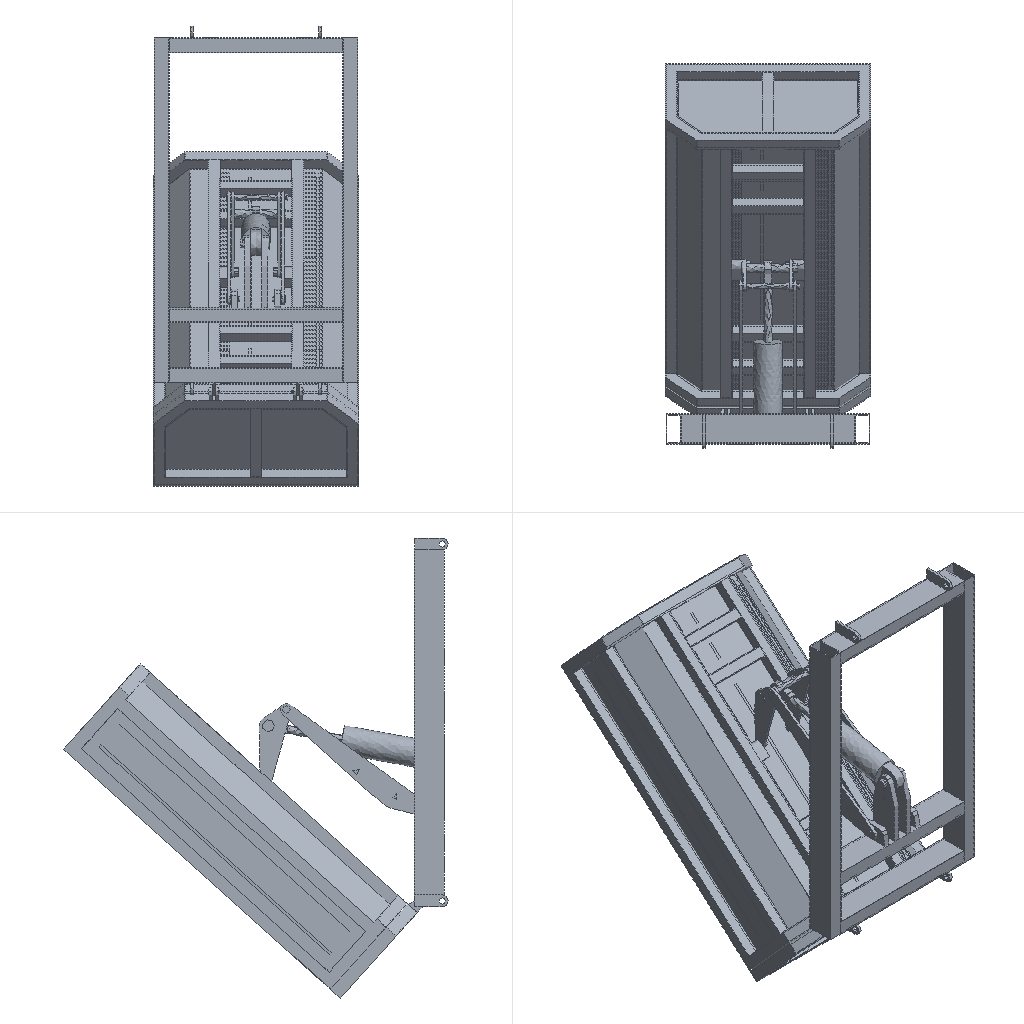Simulation study | ansys workbench
Ansys APDL input file, long lists of numbers shortened:
/batch
/config,noeldb,1     ! force off writing results to database
*get,_wallstrt,active,,time,wall
! ANSYS input file written by Workbench version 2022 R1
! File used for geometry attach:
/title,wbnew--____ (B5)
! ****** Begin Custom Load Command Snippet ******
/COM, ACT Extensions:
/COM,     LSDYNA, 2021.1
/COM,
! ****** End   Custom Load Command Snippet ******
*DIM,_wb_ProjectScratch_dir,string,248
_wb_ProjectScratch_dir(1) = ''
*DIM,_wb_SolverFiles_dir,string,248
_wb_SolverFiles_dir(1) = ''
*DIM,_wb_userfiles_dir,string,248
_wb_userfiles_dir(1) = ''
/com,--- Data in consistent NMM units. See Solving Units in the help system for more information.
/units,MPA
/nopr
/wb,file,start              !  signify a WB generated input file
/prep7
! Turn off shape checking because checks already performed inside WB mesher.
! See help system for more information.
SHPP,OFF,,NOWARN
/nolist
etcon,set             ! allow ANSYS to choose best KEYOP's for 180x elements, resets any applicable keyopt to MAPDL defaults
/com,*********** Nodes for the whole assembly ***********
nblock,3,,263278
(1i9,3e20.9e3)
        1    -2.353006712E+02    -4.029652814E+01    -6.964386465E+02
! (239343 more lines like these left out)
-1
/com,*********** Nodes for all Remote Points ***********
nblock,3
(1i9,3e20.9e3)
   239345    -1.888006686E+02     4.073828789E+02    -9.568132104E+02
-1
/wb,elem,start            !  set before creation of elements
/com,*********** Elements for Body 1 "__\____-____1" ***********
et,1,186
keyo,1,2,1          ! set full integration on SOLID186
eblock,19,solid,,8004
(19i9)
        1        1        1        1        0        0        0        0       20        0    13307    32471    32472    34084    34085    33944    33943    35521    35520
! (16007 more lines like these left out)
-1
/com,*********** Elements for Body 2 "______3c_____3e_\__________________(gb t6728-2002) 40__3(1)[6]" ***********
et,2,187
eblock,19,solid,,10404
(19i9)
        2        2        2        2        0        0        0        0       10        0     2903     6093     8090     9264     8092    10282    22392    10284    10283
! (20807 more lines like these left out)
-1
/com,*********** Elements for Body 3 "__2\____1" ***********
et,3,186
keyo,3,2,1          ! set full integration on SOLID186
eblock,19,solid,,129
(19i9)
        3        3        3        3        0        0        0        0       20        0    98906   231933   231934   231961   231960   232046   232045   232018   232019
! (257 more lines like these left out)
-1
/com,*********** Elements for Body 4 "__2\____1" ***********
et,4,186
keyo,4,2,1          ! set full integration on SOLID186
eblock,19,solid,,129
(19i9)
        4        4        4        4        0        0        0        0       20        0    99035   233038   233039   233066   233065   233151   233150   233123   233124
! (257 more lines like these left out)
-1
/com,*********** Elements for Body 5 "__28__250\____-____2" ***********
et,5,187
eblock,19,solid,,1867
(19i9)
        5        5        5        5        0        0        0        0       10        0      284      779     1143     1250     1242     2117     3926     2120     2119
! (3733 more lines like these left out)
-1
! (19 more sections like these left out)
/wb,elem,end               !  done creating elements
/com,*********** Send User Defined Coordinate System(s) ***********
csys,0
toffst,273.15,  ! Temperature offset from absolute zero
/com,*********** Set Reference Temperature ***********
tref,22.
/wb,mat,start              !  starting to send materials
/com,*********** Send Materials ***********
Temperature = 'TEMP' ! Temperature
MP,DENS,1,7.85e-09,	! tonne mm^-3
MP,ALPX,1,1.2e-05,	! C^-1
MP,C,1,434000000,	! mm^2 s^-2 C^-1
MP,KXX,1,60.5,	! tonne mm s^-3 C^-1
MP,RSVX,1,0.00017,	! ohm mm
MP,EX,1,200000,	! tonne s^-2 mm^-1
MP,NUXY,1,0.3,
MP,MURX,1,10000,
Temperature = 'TEMP' ! Temperature
MP,DENS,2,7.85e-09,	! tonne mm^-3
MP,ALPX,2,1.2e-05,	! C^-1
MP,C,2,434000000,	! mm^2 s^-2 C^-1
MP,KXX,2,60.5,	! tonne mm s^-3 C^-1
MP,RSVX,2,0.00017,	! ohm mm
MP,EX,2,200000,	! tonne s^-2 mm^-1
MP,NUXY,2,0.3,
MP,MURX,2,10000,
Temperature = 'TEMP' ! Temperature
MP,DENS,3,7.85e-09,	! tonne mm^-3
MP,ALPX,3,1.2e-05,	! C^-1
MP,C,3,434000000,	! mm^2 s^-2 C^-1
MP,KXX,3,60.5,	! tonne mm s^-3 C^-1
MP,RSVX,3,0.00017,	! ohm mm
MP,EX,3,200000,	! tonne s^-2 mm^-1
MP,NUXY,3,0.3,
MP,MURX,3,10000,
Temperature = 'TEMP' ! Temperature
MP,DENS,4,7.85e-09,	! tonne mm^-3
MP,ALPX,4,1.2e-05,	! C^-1
MP,C,4,434000000,	! mm^2 s^-2 C^-1
MP,KXX,4,60.5,	! tonne mm s^-3 C^-1
MP,RSVX,4,0.00017,	! ohm mm
MP,EX,4,200000,	! tonne s^-2 mm^-1
MP,NUXY,4,0.3,
MP,MURX,4,10000,
Temperature = 'TEMP' ! Temperature
MP,DENS,5,7.85e-09,	! tonne mm^-3
MP,ALPX,5,1.2e-05,	! C^-1
MP,C,5,434000000,	! mm^2 s^-2 C^-1
MP,KXX,5,60.5,	! tonne mm s^-3 C^-1
MP,RSVX,5,0.00017,	! ohm mm
MP,EX,5,200000,	! tonne s^-2 mm^-1
MP,NUXY,5,0.3,
MP,MURX,5,10000,
Temperature = 'TEMP' ! Temperature
MP,DENS,6,7.85e-09,	! tonne mm^-3
MP,ALPX,6,1.2e-05,	! C^-1
MP,C,6,434000000,	! mm^2 s^-2 C^-1
MP,KXX,6,60.5,	! tonne mm s^-3 C^-1
MP,RSVX,6,0.00017,	! ohm mm
MP,EX,6,200000,	! tonne s^-2 mm^-1
MP,NUXY,6,0.3,
MP,MURX,6,10000,
Temperature = 'TEMP' ! Temperature
MP,DENS,7,7.85e-09,	! tonne mm^-3
MP,ALPX,7,1.2e-05,	! C^-1
MP,C,7,434000000,	! mm^2 s^-2 C^-1
MP,KXX,7,60.5,	! tonne mm s^-3 C^-1
MP,RSVX,7,0.00017,	! ohm mm
MP,EX,7,200000,	! tonne s^-2 mm^-1
MP,NUXY,7,0.3,
MP,MURX,7,10000,
Temperature = 'TEMP' ! Temperature
MP,DENS,8,7.85e-09,	! tonne mm^-3
MP,ALPX,8,1.2e-05,	! C^-1
MP,C,8,434000000,	! mm^2 s^-2 C^-1
MP,KXX,8,60.5,	! tonne mm s^-3 C^-1
MP,RSVX,8,0.00017,	! ohm mm
MP,EX,8,200000,	! tonne s^-2 mm^-1
MP,NUXY,8,0.3,
MP,MURX,8,10000,
Temperature = 'TEMP' ! Temperature
MP,DENS,9,7.85e-09,	! tonne mm^-3
MP,ALPX,9,1.2e-05,	! C^-1
MP,C,9,434000000,	! mm^2 s^-2 C^-1
MP,KXX,9,60.5,	! tonne mm s^-3 C^-1
MP,RSVX,9,0.00017,	! ohm mm
MP,EX,9,200000,	! tonne s^-2 mm^-1
! (137 more lines like these left out)
/wb,mat,end                !  done sending materials
!************************* Model Summary ********************
!__\____-____1,	结构钢,	matid,	1
!______3c_____3e_\__________________(gb t6728-2002) 40__3(1)[6],	结构钢,	matid,	2
!__2\____1,	结构钢,	matid,	3
!__2\____1,	结构钢,	matid,	4
!__28__250\____-____2,	结构钢,	matid,	5
!__3\____-____5,	结构钢,	matid,	6
!__3\____-____5,	结构钢,	matid,	7
!__1\____-____1,	结构钢,	matid,	8
!__1\____-____1,	结构钢,	matid,	9
!________3c_____3e_\__________________gb_Mt6728-2002 100__50__3(1)[2],	结构钢,	matid,	10
!____1\____1,	结构钢,	matid,	11
!____1\____1,	结构钢,	matid,	12
!____2\______1,	结构钢,	matid,	13
!____2\______1,	结构钢,	matid,	14
!M30X90\____-____1,	结构钢,	matid,	15
!M20X40__\____-____1,	结构钢,	matid,	16
!M20X40__\____-____1,	结构钢,	matid,	17
!M20X200__\____-____1,	结构钢,	matid,	18
!M30X180__\____-____1,	结构钢,	matid,	19
!M20X20-16____\____1,	结构钢,	matid,	20
!M20X20-16____\____1,	结构钢,	matid,	21
!M12X38__\____-____1,	结构钢,	matid,	22
!M12X38__\____-____1,	结构钢,	matid,	23
!______3c_____3e_\__________________(gb t6728-2002) 40__3(1)[1],	结构钢,	matid,	24
!************************* End Model Summary ********************
! get the diagonal of the bounding box. Needed later for other things
*get,_xmin,node,,mnloc,x
*get,_ymin,node,,mnloc,y
*get,_zmin,node,,mnloc,z
*get,_xmax,node,,mxloc,x
*get,_ymax,node,,mxloc,y
*get,_zmax,node,,mxloc,z
_ASMDIAG=(_xmax-_xmin)*(_xmax-_xmin)+(_ymax-_ymin)*(_ymax-_ymin)+(_zmax-_zmin)*(_zmax-_zmin)
_ASMDIAG=SQRT(_ASMDIAG)
/wb,contact,start          !  starting to send contact
/com,*********** Create Contact "接触区域" ***********
/com,            Real Constant Set For Above Contact Is 26 & 25
*set,tid,26
*set,cid,25
r,tid
r,cid
et,tid,170
et,cid,174
eblock,10,,,138
(15i9)
   176923       26       26       26        0    33942    35521    33943    33943    64183    64185    33943    64182
! (137 more lines like these left out)
-1
eblock,10,,,138
(15i9)
   177061       25       25       25        0    33942    35521    33943    33943    64183    64185    33943    64182
! (137 more lines like these left out)
-1
eblock,10,,,162
(15i9)
   177199       25       26       25        0     8144     8214     8175     8175    22993    23314     8175    22991
! (161 more lines like these left out)
-1
eblock,10,,,162
(15i9)
   177361       26       25       26        0     8144     8214     8175     8175    22993    23314     8175    22991
! (161 more lines like these left out)
-1
keyo,cid,8,2               ! auto create asymmetric contact (from Program Controlled setting)
keyo,cid,10,0              ! adjust contact stiffness each NR iteration (from Program Controlled setting)
keyo,cid,12,5              ! bonded always
keyo,cid,2,2               ! MPC contact.  Valid only for bonded or no separation.  Requires nodal detection
keyo,cid,4,2               ! on nodal point - normal to target surface (from Program Controlled setting)
keyo,cid,9,1               ! ignore initial gaps/penetration
keyo,cid,7,0               ! No Prediction
rmod,tid,3,10.      ! FKN
rmod,tid,5,0.       ! ICONT
rmod,tid,6,-5.      ! PINB
rmod,tid,10,0.      ! CNOF
rmod,tid,12,0.      ! FKT
rmod,tid,36,95      ! WB DSID
rmod,cid,3,10.      ! FKN
rmod,cid,5,0.       ! ICONT
rmod,cid,6,-5.      ! PINB
rmod,cid,10,0.      ! CNOF
rmod,cid,12,0.      ! FKT
rmod,cid,36,95      ! WB DSID
/com,*********** Create Contact "接触区域 8" ***********
/com,            Real Constant Set For Above Contact Is 28 & 27
*set,tid,28
*set,cid,27
r,tid
r,cid
et,tid,170
et,cid,174
eblock,10,,,3771
(15i9)
   177523       28       28       28        0    28251    26712    26655    26654    41903    41789    41786    41787
! (3770 more lines like these left out)
-1
eblock,10,,,3771
(15i9)
   181294       27       27       27        0    28251    26712    26655    26654    41903    41789    41786    41787
! (3770 more lines like these left out)
-1
eblock,10,,,3247
(15i9)
   185065       27       28       27        0   139835   149281   144474   144474   166900   201084   144474   166896
! (3246 more lines like these left out)
-1
eblock,10,,,3247
(15i9)
   188312       28       27       28        0   139835   149281   144474   144474   166900   201084   144474   166896
! (3246 more lines like these left out)
-1
keyo,cid,8,2               ! auto create asymmetric contact (from Program Controlled setting)
keyo,cid,10,0              ! adjust contact stiffness each NR iteration (from Program Controlled setting)
keyo,cid,12,5              ! bonded always
keyo,cid,2,2               ! MPC contact.  Valid only for bonded or no separation.  Requires nodal detection
keyo,cid,4,2               ! on nodal point - normal to target surface (from Program Controlled setting)
keyo,cid,9,1               ! ignore initial gaps/penetration
keyo,cid,7,0               ! No Prediction
rmod,tid,3,10.      ! FKN
rmod,tid,5,0.       ! ICONT
rmod,tid,6,-5.      ! PINB
rmod,tid,10,0.      ! CNOF
rmod,tid,12,0.      ! FKT
rmod,tid,36,116     ! WB DSID
rmod,cid,3,10.      ! FKN
rmod,cid,5,0.       ! ICONT
rmod,cid,6,-5.      ! PINB
rmod,cid,10,0.      ! CNOF
rmod,cid,12,0.      ! FKT
rmod,cid,36,116     ! WB DSID
/com,*********** Create Contact "接触区域 11" ***********
/com,            Real Constant Set For Above Contact Is 30 & 29
*set,tid,30
*set,cid,29
r,tid
r,cid
et,tid,170
et,cid,174
eblock,10,,,54
(15i9)
   191559       30       30       30        0     6070     6066     6058     6058    10162    10117     6058    10118
! (53 more lines like these left out)
-1
eblock,10,,,54
(15i9)
   191613       29       29       29        0     6070     6066     6058     6058    10162    10117     6058    10118
! (53 more lines like these left out)
-1
eblock,10,,,96
(15i9)
   191667       29       30       29        0   238922   238921   238955   238955   239014   239016   238955   239019
! (95 more lines like these left out)
-1
eblock,10,,,96
(15i9)
   191763       30       29       30        0   238922   238921   238955   238955   239014   239016   238955   239019
! (95 more lines like these left out)
-1
keyo,cid,8,2               ! auto create asymmetric contact (from Program Controlled setting)
keyo,cid,10,0              ! adjust contact stiffness each NR iteration (from Program Controlled setting)
keyo,cid,12,5              ! bonded always
keyo,cid,2,2               ! MPC contact.  Valid only for bonded or no separation.  Requires nodal detection
keyo,cid,4,2               ! on nodal point - normal to target surface (from Program Controlled setting)
keyo,cid,9,1               ! ignore initial gaps/penetration
keyo,cid,7,0               ! No Prediction
rmod,tid,3,10.      ! FKN
rmod,tid,5,0.       ! ICONT
rmod,tid,6,-5.      ! PINB
rmod,tid,10,0.      ! CNOF
rmod,tid,12,0.      ! FKT
rmod,tid,36,125     ! WB DSID
rmod,cid,3,10.      ! FKN
rmod,cid,5,0.       ! ICONT
rmod,cid,6,-5.      ! PINB
rmod,cid,10,0.      ! CNOF
rmod,cid,12,0.      ! FKT
rmod,cid,36,125     ! WB DSID
/com,*********** Create Contact "接触区域 12" ***********
/com,            Real Constant Set For Above Contact Is 32 & 31
*set,tid,32
*set,cid,31
r,tid
r,cid
et,tid,170
et,cid,174
eblock,10,,,201
(15i9)
   191859       32       32       32        0     8144     8214     8175     8175    22993    23314     8175    22991
! (200 more lines like these left out)
-1
eblock,10,,,201
(15i9)
   192060       31       31       31        0     8144     8214     8175     8175    22993    23314     8175    22991
! (200 more lines like these left out)
-1
eblock,10,,,428
(15i9)
   192261       31       32       31        0   138273   149145   149139   149139   154407   222313   149139   154406
! (427 more lines like these left out)
-1
eblock,10,,,428
(15i9)
   192689       32       31       32        0   138273   149145   149139   149139   154407   222313   149139   154406
! (427 more lines like these left out)
-1
keyo,cid,8,2               ! auto create asymmetric contact (from Program Controlled setting)
keyo,cid,10,0              ! adjust contact stiffness each NR iteration (from Program Controlled setting)
keyo,cid,12,5              ! bonded always
keyo,cid,2,2               ! MPC contact.  Valid only for bonded or no separation.  Requires nodal detection
keyo,cid,4,2               ! on nodal point - normal to target surface (from Program Controlled setting)
keyo,cid,9,1               ! ignore initial gaps/penetration
keyo,cid,7,0               ! No Prediction
rmod,tid,3,10.      ! FKN
rmod,tid,5,0.       ! ICONT
rmod,tid,6,-5.      ! PINB
rmod,tid,10,0.      ! CNOF
rmod,tid,12,0.      ! FKT
rmod,tid,36,128     ! WB DSID
rmod,cid,3,10.      ! FKN
rmod,cid,5,0.       ! ICONT
rmod,cid,6,-5.      ! PINB
rmod,cid,10,0.      ! CNOF
rmod,cid,12,0.      ! FKT
rmod,cid,36,128     ! WB DSID
/com,*********** Create Contact "接触区域 15" ***********
/com,            Real Constant Set For Above Contact Is 34 & 33
*set,tid,34
*set,cid,33
r,tid
r,cid
et,tid,170
et,cid,174
eblock,10,,,23
(15i9)
   193117       34       34       34        0   232168   232149   232143   232167   232893   232880   232881   232925
! (22 more lines like these left out)
-1
eblock,10,,,23
(15i9)
   193140       33       33       33        0   232168   232149   232143   232167   232893   232880   232881   232925
! (22 more lines like these left out)
-1
eblock,10,,,48
(15i9)
   193163       33       34       33        0   237237   237258   237253   237253   237535   237602   237253   237534
! (47 more lines like these left out)
-1
eblock,10,,,48
(15i9)
   193211       34       33       34        0   237237   237258   237253   237253   237535   237602   237253   237534
! (47 more lines like these left out)
-1
keyo,cid,8,2               ! auto create asymmetric contact (from Program Controlled setting)
keyo,cid,10,0              ! adjust contact stiffness each NR iteration (from Program Controlled setting)
keyo,cid,12,5              ! bonded always
keyo,cid,2,2               ! MPC contact.  Valid only for bonded or no separation.  Requires nodal detection
keyo,cid,4,2               ! on nodal point - normal to target surface (from Program Controlled setting)
keyo,cid,9,1               ! ignore initial gaps/penetration
keyo,cid,7,0               ! No Prediction
rmod,tid,3,10.      ! FKN
rmod,tid,5,0.       ! ICONT
rmod,tid,6,-5.      ! PINB
rmod,tid,10,0.      ! CNOF
rmod,tid,12,0.      ! FKT
rmod,tid,36,137     ! WB DSID
rmod,cid,3,10.      ! FKN
rmod,cid,5,0.       ! ICONT
rmod,cid,6,-5.      ! PINB
rmod,cid,10,0.      ! CNOF
rmod,cid,12,0.      ! FKT
rmod,cid,36,137     ! WB DSID
! (25 more sections like these left out)
/wb,contact,end            !  done creating contacts
/golist
/wb,load,start             !  starting to send loads
/com,*********** Fixed Supports ***********
CMBLOCK,_FIXEDSU,NODE,      348
(8i10)
     78153     78154     78155     78156     78157     78158     78285     78286
! (43 more lines like these left out)
cmsel,s,_FIXEDSU
d,all,all
nsel,all
/com,*********** Create Remote Point "内部远程点" ***********
! -------- Remote Point Used by "点质量" --------
*set,tid,86
*set,cid,85
et,cid,174
et,tid,170
keyo,tid,2,1               ! Don't fix the pilot node
keyo,tid,4,000111
keyo,cid,12,5              ! Bonded Contact
keyo,cid,4,3               ! Coupled CPINTF style load
keyo,cid,2,2               ! MPC style contact
eblock,10,,,4455
(15i9)
   197199       85       85       85        0    38777    36282    38775    38776    68825    68824    73766    73767
! (4454 more lines like these left out)
-1
*set,_npilot,239345
_npilot246=_npilot
type,tid
mat ,cid
real,cid
tshape,pilo
en,201654,_npilot
tshape
/com,*********** Construct Remote Mass Using Remote Attachment ***********
*set,_tid,87
et,_tid,21           ! MASS21 element
type,_tid
mat ,_tid
real,_tid
keyo,_tid,3,2        ! 3d mass without rotary inertia
r,_tid,0.5
en,201655,239345
/gst,on,on
fini
*get,_numnode,node,0,count
*get,_numelem,elem,0,count
*get, _MAXELEMNUM, elem, 0, NUM, MAX
*get, _MAXNODENUM, node, 0, NUM, MAX
*get, _MAXELEMTYPE, etyp, 0, NUM, MAX
*get, _MAXREALCONST, real, 0, NUM, MAX
/go
/wb,load,end               !  done creating loads
/com,--- Number of total nodes = %_numnode%
/com,--- Number of contact elements = 24731
/com,--- Number of spring elements = 0
/com,--- Number of bearing elements = 0
/com,--- Number of solid elements = 100731
/com,--- Number of condensed parts = 0
/com,--- Number of total elements = %_numelem%
*get,_wallbsol,active,,time,wall
/com,****************************************************************************
/com,*************************    SOLUTION       ********************************
/com,****************************************************************************
/solu
antype,0                   ! static analysis
neqit,1,force              ! Force 1 eq iteration since only nonlinearity is bonded/no sep contact
pred,off
_thickRatio=0.208   ! Ratio of thick parts in the model
eqsl,sparse,,,,,1
cntr,print,1               ! print out contact info and also make no initial contact an error
dmpoption,emat,no             ! Don't combine emat file for DANSYS
dmpoption,esav,no             ! Don't combine esav file for DANSYS
nldiag,cont,iter           ! print out contact info each equilibrium iteration
rescontrol,,none                 ! Do not keep any restart files
/com,****************************************************
/com,******************* SOLVE FOR LS 1 OF 1 ****************
acel,0.,9806.65,0.
/nopr
/gopr
nsub,1,1,1
time,1.
outres,erase
outres,all,none
outres,nsol,all,
outres,rsol,all
outres,eangl,all
outres,etmp,all
outres,veng,all
outres,strs,all,
outres,epel,all,
outres,eppl,all,
outres,cont,all,
! *********** WB SOLVE COMMAND ***********
! check interactive state
*get,ANSINTER_,active,,int
*if,ANSINTER_,ne,0,then
/eof
*endif
solve
/com *************** Write FE CONNECTORS *********
CEWRITE,file,ce,,INTE
/com,****************************************************
/com,*************** FINISHED SOLVE FOR LS 1 *************
*get,_wallasol,active,,time,wall
/nopr
*get,_numnode,node,0,count
*get,_numelem,elem,0,count
*get, _MAXELEMNUM, elem, 0, NUM, MAX
*get, _MAXNODENUM, node, 0, NUM, MAX,,,INTERNAL
*get, _MAXELEMTYPE, etyp, 0, NUM, MAX
*get, _MAXREALCONST, real, 0, NUM, MAX
/gopr
/post1
xmlo,ENCODING,ISO-8859-1
xmlo,parm
/xml,parm,xml
fini
/gopr
*get,_walldone,active,,time,wall
_preptime=(_wallbsol-_wallstrt)*3600
_solvtime=(_wallasol-_wallbsol)*3600
_posttime=(_walldone-_wallasol)*3600
_totaltim=(_walldone-_wallstrt)*3600
*get,_dlbratio,active,0,solu,dlbr
*get,_combtime,active,0,solu,comb
*get,_ssmode,active,0,solu,ssmm
*get,_ndofs,active,0,solu,ndof
*get,_sol_end_time,active,0,set,time
*if,_sol_end_time,eq,1.,then
/fclean				!clean distributed files
*endif
/com,--- Total number of nodes = %_numnode%
/com,--- Total number of elements = %_numelem%
/com,--- Element load balance ratio = %_dlbratio%
/com,--- Time to combine distributed files = %_combtime%
/com,--- Sparse memory mode = %_ssmode%
/com,--- Number of DOF = %_ndofs%
/wb,file,end               ! done with WB generated input